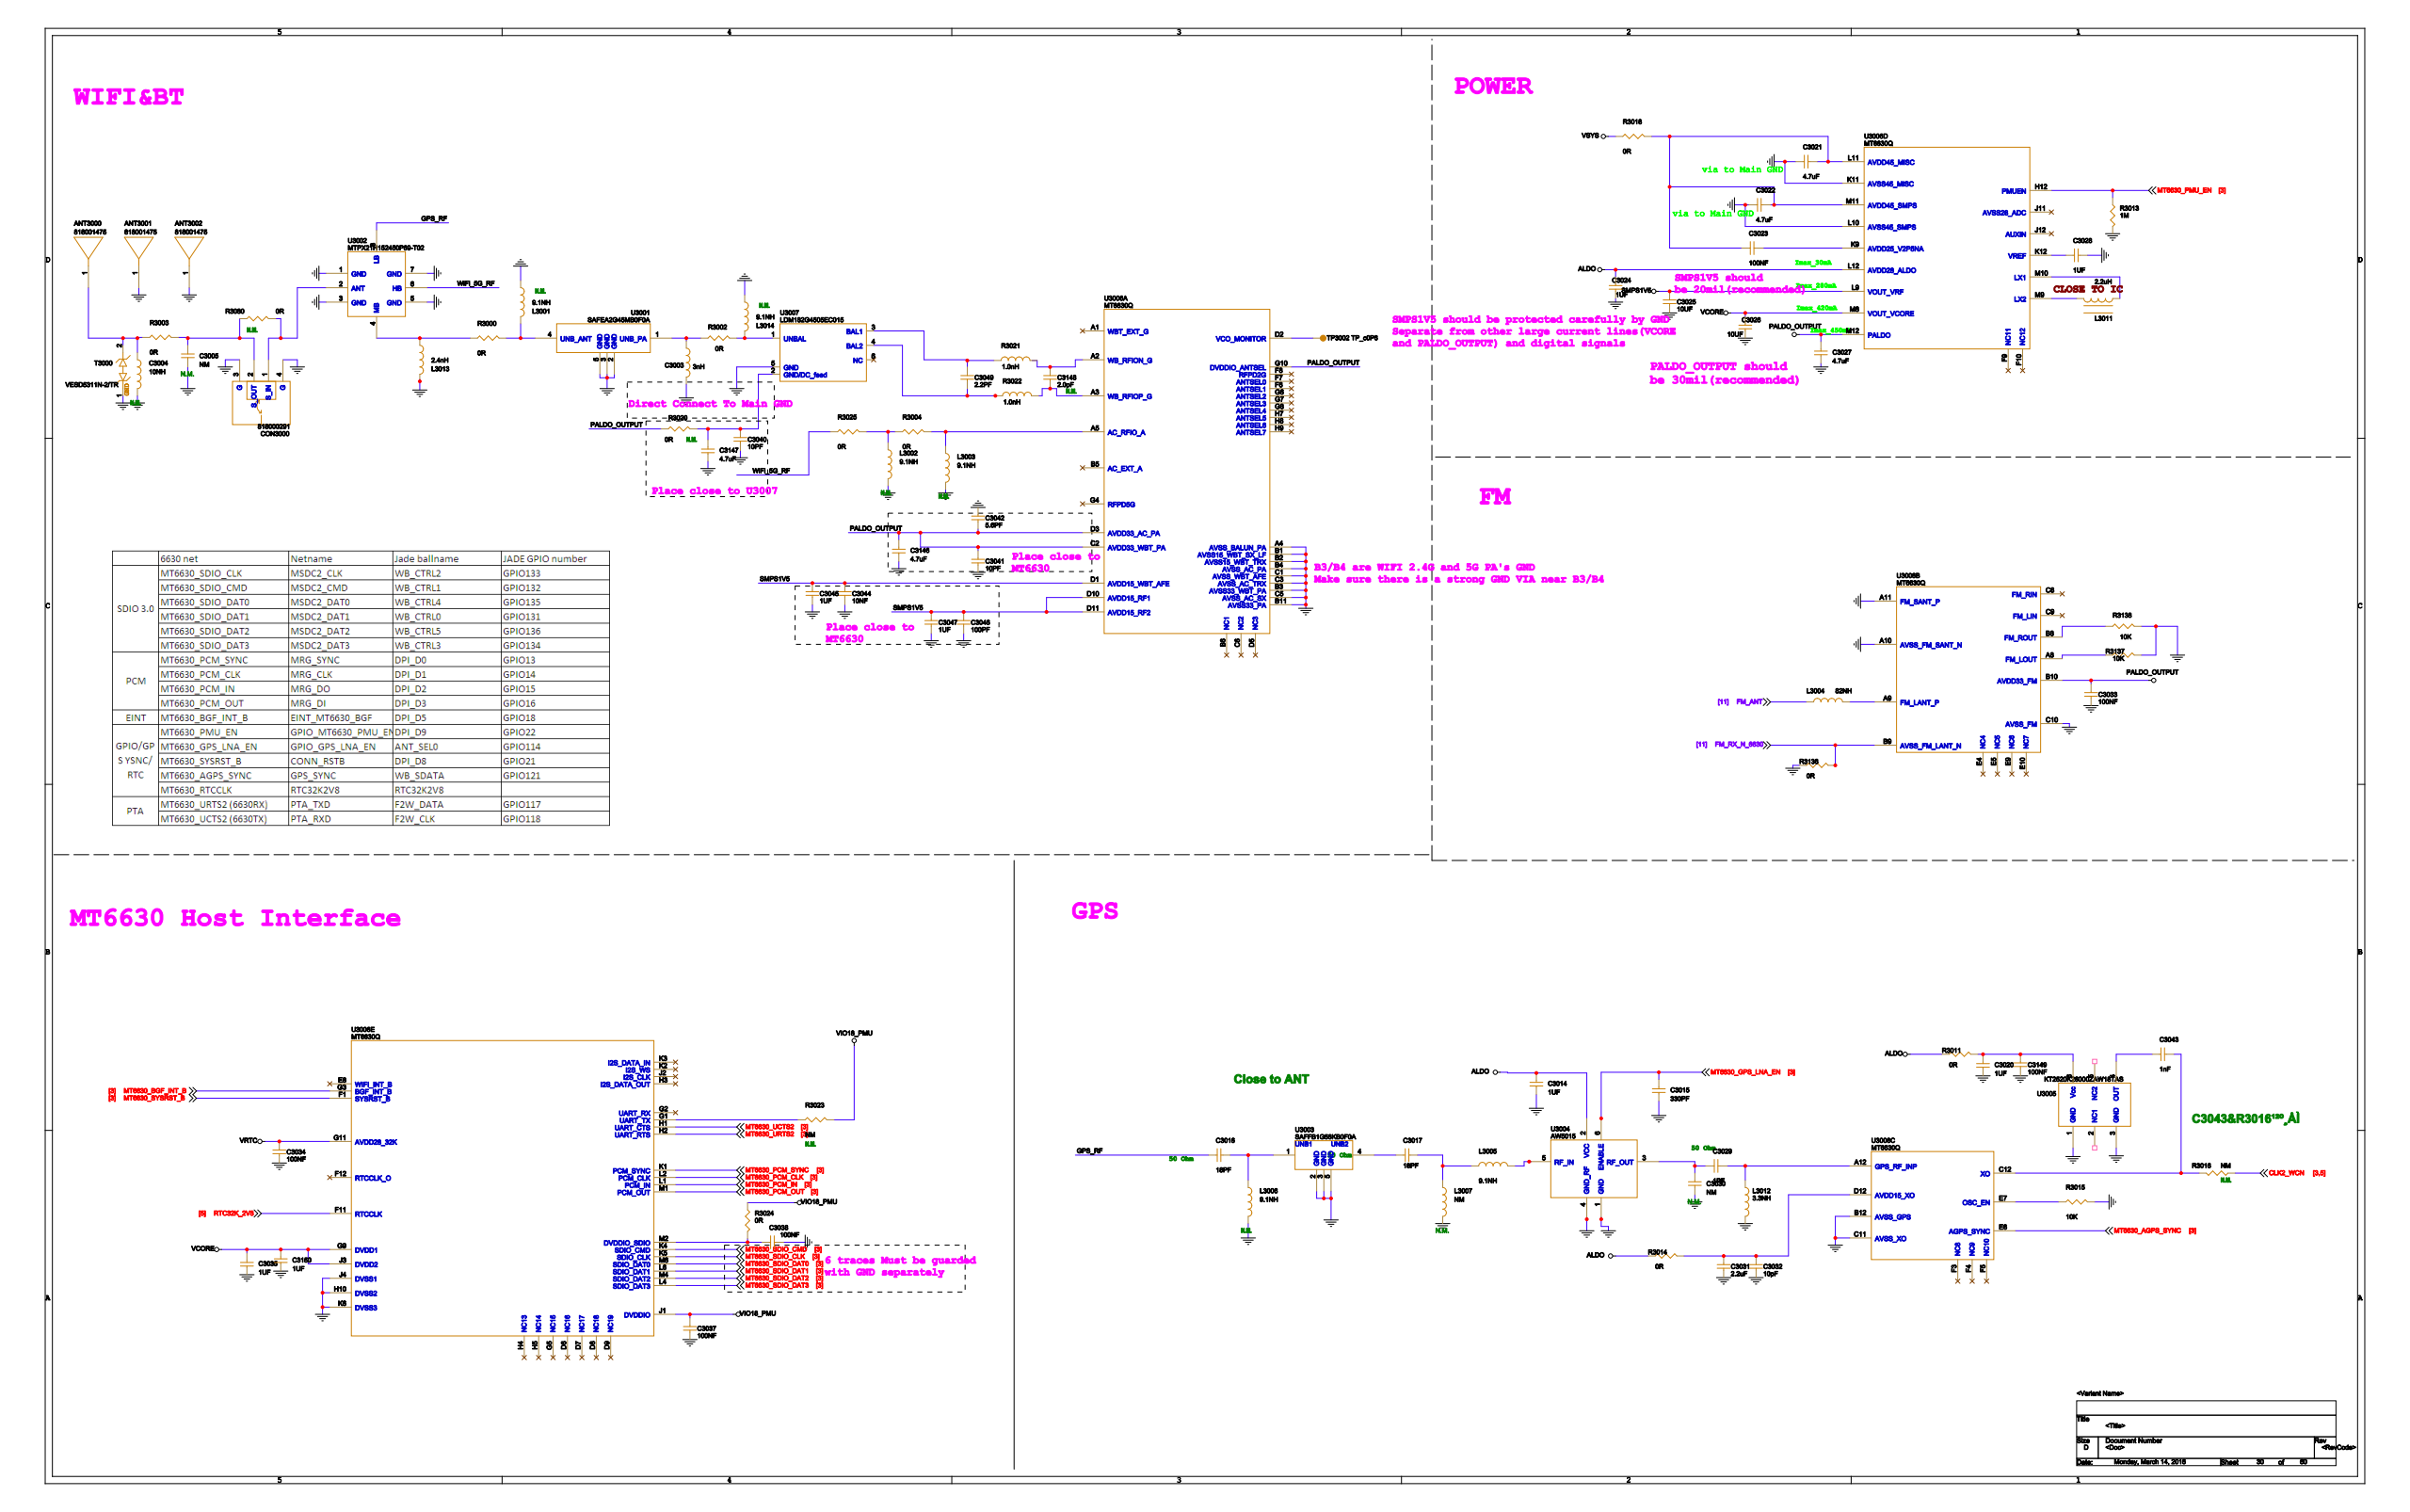Circuit board | Cadence Allegro | 1088 parts | 793 nets | one sheet of the schematic
Parts on this sheet (reference | value | footprint):
ANT3000 | 818001475 | PIN_ANT_818001475
ANT3001 | 818001475 | PIN_ANT_818001475
ANT3002 | 818001475 | PIN_ANT_818001475
C3003 | 3nH | L0201
C3004
C3005
C3014 | 1UF | C0201
C3015 | 330PF | C0201
C3016 | 18PF | C0201
C3017 | 18PF | C0201
C3020 | 1UF | C0201
C3021 | 4.7uF | 0402-BIG
C3022 | 4.7uF | 0402-BIG
C3023 | 100NF | C0201
C3024 | 1UF | C0201
C3025 | 10UF | 0603-BIG
C3026 | 10UF | 0603-BIG
C3027 | 4.7uF | 0402-BIG
C3028 | 1UF | C0201
C3029 | 1PF | C0201
C3030
C3031 | 2.2uF | C0201
C3032 | 10PF | C0201
C3033 | 100NF | C0201
C3034 | 100NF | C0201
C3035 | 1UF | C0201
C3037 | 100NF | C0201
C3038 | 100NF | C0201
C3040 | 10PF | C0201
C3041 | 10PF | C0201
C3042 | 5.6PF | C0201
C3043 | 1nF | C0201
C3044 | 10nF | C0201
C3045 | 1UF | C0201
C3046 | 100PF | C0201
C3047 | 1UF | C0201
C3049 | 2.2PF | C0201
C3146 | 4.7uF | 0402-BIG
C3147 | 4.7uF | 0402-BIG
C3148
C3149 | 100NF | C0201
C3150 | 1UF | C0201
CON3000 | 818000291 | RF_818000291
L3001
L3002
L3003
L3004 | 82NH | L0402
L3005 | 9.1NH | L0201
L3006
L3007
L3011 | 2.2uH | L2520_VLS252010CX
L3012 | 3.3NH | L0201
L3013 | 2.4nH | L0201
L3014
R3000 | 0R | R0201
R3002 | 0R | R0201
R3003 | 0R | R0201
R3004 | 0R | R0201
R3011 | 0R | R0201
R3013 | 1M | R0201
R3014 | 0R | R0201
R3015 | 10K | R0201
R3016
R3018 | 0R | R0402
R3020
R3021 | 1.0nH | L0201
R3022 | 1.0nH | L0201
R3023
R3024 | 0R | R0201
R3025 | 0R | R0201
R3080
R3136 | 0R | R0201
R3137 | 10K | R0201
R3138 | 10K | R0201
T3000 | VESD5311N-2/TR | DFN1006-2
TP3002 | TP_c0P6 | TP_C0P6
U3001 | SAFEA2G45MB0F0A | SAW1411_H0P6_MURATA
U3002 | MTPX21H152450P69-T02 | MTPX21
U3003 | SAFFB1G56KB0F0A | SAW1109_H0P6_MURATA
U3004 | AW5015 | DFN6_0P9X1P1X0P6_0P4
U3005 | KT2520K26000ZAW18TAS | KT2520F
U3006 | MT6630Q | MT6630Q
U3007 | LDM182G4505EC015 | LDM182G4505EC015
Nets of these parts (net: part-pin ...):
GND: ANT3001-1 ANT3002-1 C3003-2 C3004-2 C3005-2 C3014-1 C3015-1 C3020-1 C3021-1 C3022-1 C3024-2 C3025-2 C3026-2 C3027-1 C3028-2 C3030-2 C3031-2 C3032-2 C3033-2 C3034-2 C3035-1 C3037-2 C3038-2 C3040-2 C3041-2 C3042-1 C3044-2 C3045-2 C3046-2 C3047-2 C3146-1 C3147-1 C3149-2 C3150-1 CON3000-3 CON3000-4 L3001-2 L3002-2 L3003-2 L3006-2 L3007-2 L3012-2 L3013-1 L3014-2 R3013-2 R3015-2 R3136-1 R3137-2 R3138-2 T3000-1 U3001-2 U3001-3 U3001-5 U3002-1 U3002-3 U3002-5 U3002-7 U3003-2 U3003-3 U3003-5 U3004-1 U3004-4 U3005-1 U3005-3 U3007-5 U3006-A4 U3006-A10 U3006-A11 U3006-B1 U3006-B2 U3006-B3 U3006-B4 U3006-B11 U3006-B12 U3006-C1 U3006-C3 U3006-C5 U3006-C10 U3006-C11 U3006-H10 U3006-J4 U3006-K6 U3006-K11 U3006-L10
N34496068: C3003-1 R3002-1 U3001-1
N34495988: C3049-1 R3021-1 U3007-3
N34495991: C3049-2 R3022-1 U3007-4
N34460109: L3013-2 R3000-1 U3002-4
N34460906: C3148-1 R3021-2 U3006-A2
N34460895: C3148-2 R3022-2 U3006-A3
VSYS: R3018-1
N34495838: CON3000-1 R3080-2 U3002-2
N34495825: C3005-1 CON3000-2 R3003-2 R3080-1
N34496067: L3001-1 R3000-2 U3001-4
N35478653: C3016-2 L3006-1 U3003-1
N35479079: C3017-2 U3003-4
MT6630_GPS_LNA_EN: C3015-2 U3004-6
N35478657: L3005-2 U3004-5
N35478681: C3029-1 C3030-1 U3004-3
ALDO: C3014-2 C3024-1 R3011-1 R3014-1 U3004-2 U3006-L12
N35478675: C3043-1 U3005-4
N35478671: C3020-2 C3149-1 R3011-2 U3005-6
N34495831: ANT3000-1 C3004-1 R3003-1 T3000-2
MT6630_PCM_SYNC: U3006-K1
MT6630_PCM_CLK: U3006-L2
MT6630_PCM_IN: U3006-L1
MT6630_PCM_OUT: U3006-M1
MT6630_BGF_INT_B: U3006-G3
MT6630_SYSRST_B: U3006-F1
MT6630_PMU_EN: R3013-1 U3006-H12
MT6630_UCTS2: U3006-H1
MT6630_URTS2: U3006-H2
MT6630_SDIO_DAT1: U3006-L6
MT6630_SDIO_CMD: U3006-K4
MT6630_SDIO_CLK: U3006-K5
MT6630_SDIO_DAT3: U3006-L4
MT6630_SDIO_DAT0: U3006-M6
MT6630_SDIO_DAT2: U3006-M4
MT6630_AGPS_SYNC: U3006-E6
VIO18_PMU: C3037-1 R3023-2 R3024-1 U3006-J1
PALDO_OUTPUT: C3027-2 C3033-1 C3041-1 C3042-2 C3146-2 R3020-1 U3006-B10 U3006-C2 U3006-D3 U3006-G10 U3006-M12
N34495921: L3011-1 U3006-M10
N34495920: L3011-2 U3006-M9
WIFI_5G_RF: R3025-1 U3002-6
GPS_RF: C3016-1 U3002-8
N34496056: L3003-1 R3004-2 U3006-A5
SMPS1V5: C3025-1 C3044-1 C3045-1 C3046-1 C3047-1 U3006-D1 U3006-D10 U3006-D11 U3006-L9
N34496050: TP3002-1 U3006-D2
FM_RX_N_6630: R3136-2 U3006-B9
N34495944: L3004-2 U3006-A9
N35031005: R3137-1 U3006-A8
N35031013: R3138-1 U3006-B8
N35478691: C3031-1 C3032-1 R3014-2 U3006-D12
N35478640: C3029-2 L3012-1 U3006-A12
N35478715: R3015-1 U3006-E7
N35478677: C3043-2 R3016-2 U3006-C12
N34495900: C3023-2 U3006-K9
N34495881: C3021-2 C3022-2 C3023-1 R3018-2 U3006-L11 U3006-M11
VCORE: C3026-1 C3035-2 C3150-2 U3006-G9 U3006-J3 U3006-M8
N34495918: C3028-1 U3006-K12
VRTC: C3034-1 U3006-G11
N34495978: C3038-1 R3024-2 U3006-M2
RTC32K_2V8: U3006-F11
N34496051: R3023-1 U3006-G1
N34495996: C3040-1 C3147-2 R3020-2 U3007-2
N34460758: L3014-1 R3002-2 U3007-1
CLK2_WCN: R3016-1
N35478632: C3017-1 L3005-1 L3007-1
N34496055: L3002-1 R3004-1 R3025-2
FM_ANT: L3004-1